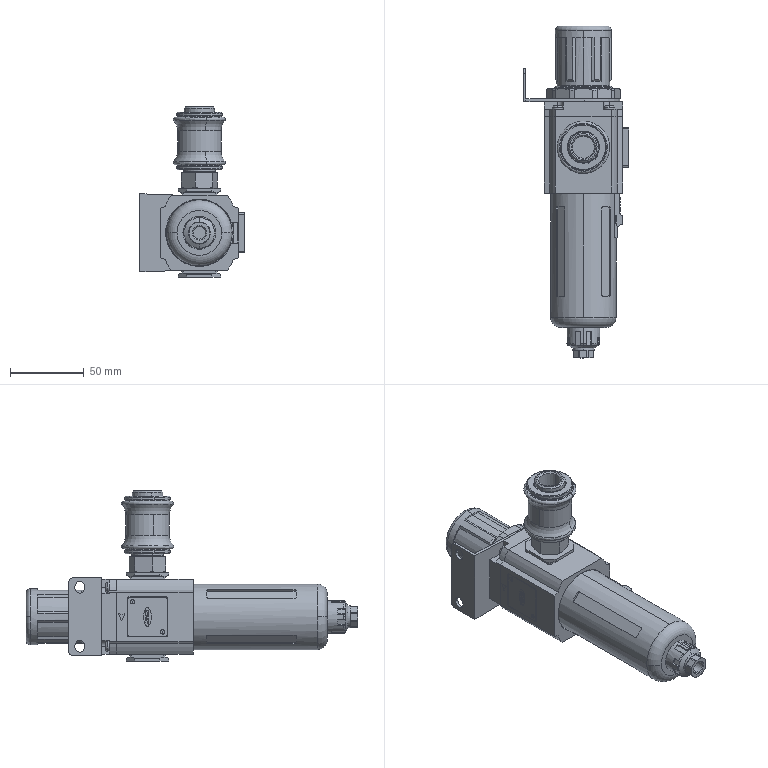Part | SolidWorks | 20 solids | 1192 faces | box 72 x 225.5 x 115.5 mm | volume 326380 mm3 | plane 706 | cylinder 339 | cone 77 | torus 70 | commonest cylinder face diameters 4 x43 2 x34 3 x18 40 x14 7 x12 50 x11